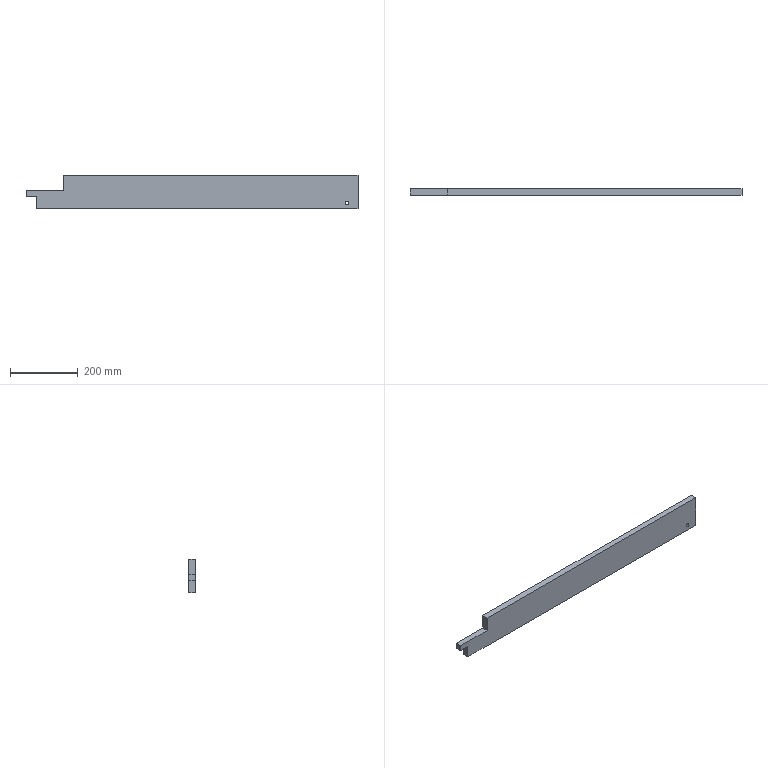Part | STEP file | Superstructure_3 | 1 solid | 11 faces | box 980 x 18 x 100 mm | volume 1653506 mm3 | plane 10 | cylinder 1 | commonest cylinder face diameters 10 x1
STEP:
#1=CARTESIAN_POINT('',(0.,0.,0.));
#2=DIRECTION('',(0.,0.,1.));
#3=DIRECTION('',(1.,0.,0.));
#4=AXIS2_PLACEMENT_3D('',#1,#2,#3);
#5=CARTESIAN_POINT('',(0.,9.,0.));
#6=VERTEX_POINT('',#5);
#7=CARTESIAN_POINT('',(0.,-9.,0.));
#8=VERTEX_POINT('',#7);
#9=CARTESIAN_POINT('',(0.,9.,0.));
#10=DIRECTION('',(0.,-1.,0.));
#11=VECTOR('',#10,1.);
#12=LINE('',#9,#11);
#13=CARTESIAN_POINT('',(0.,9.,0.));
#14=DIRECTION('',(-1.,0.,0.));
#15=DIRECTION('',(0.,0.,1.));
#16=AXIS2_PLACEMENT_3D('',#13,#14,#15);
#17=PLANE('',#16);
#18=CARTESIAN_POINT('',(0.,0.));
#19=DIRECTION('',(0.,-1.));
#20=VECTOR('',#19,1.);
#21=LINE('',#18,#20);
#22=(GEOMETRIC_REPRESENTATION_CONTEXT(2)PARAMETRIC_REPRESENTATION_CONTEXT()REPRESENTATION_CONTEXT('',''));
#23=DEFINITIONAL_REPRESENTATION('',(#21),#22);
#24=PCURVE('',#17,#23);
#25=CARTESIAN_POINT('',(950.,9.,0.));
#26=DIRECTION('',(0.,0.,-1.));
#27=DIRECTION('',(-1.,0.,0.));
#28=AXIS2_PLACEMENT_3D('',#25,#26,#27);
#29=PLANE('',#28);
#30=CARTESIAN_POINT('',(950.,0.));
#31=DIRECTION('',(0.,-1.));
#32=VECTOR('',#31,1.);
#33=LINE('',#30,#32);
#34=(GEOMETRIC_REPRESENTATION_CONTEXT(2)PARAMETRIC_REPRESENTATION_CONTEXT()REPRESENTATION_CONTEXT('',''));
#35=DEFINITIONAL_REPRESENTATION('',(#33),#34);
#36=PCURVE('',#29,#35);
#37=SURFACE_CURVE('',#12,(#24,#36),.PCURVE_S1.);
#38=EDGE_CURVE('',#6,#8,#37,.T.);
#39=ORIENTED_EDGE('',*,*,#38,.T.);
#40=CARTESIAN_POINT('',(0.,-9.,37.));
#41=VERTEX_POINT('',#40);
#42=CARTESIAN_POINT('',(0.,-9.,0.));
#43=DIRECTION('',(0.,0.,1.));
#44=VECTOR('',#43,1.);
#45=LINE('',#42,#44);
#46=CARTESIAN_POINT('',(0.,-18.));
#47=DIRECTION('',(1.,0.));
#48=VECTOR('',#47,1.);
#49=LINE('',#46,#48);
#50=(GEOMETRIC_REPRESENTATION_CONTEXT(2)PARAMETRIC_REPRESENTATION_CONTEXT()REPRESENTATION_CONTEXT('',''));
#51=DEFINITIONAL_REPRESENTATION('',(#49),#50);
#52=PCURVE('',#17,#51);
#53=CARTESIAN_POINT('',(468.21,-9.,47.857));
#54=DIRECTION('',(0.,1.,0.));
#55=DIRECTION('',(0.,0.,1.));
#56=AXIS2_PLACEMENT_3D('',#53,#54,#55);
#57=PLANE('',#56);
#58=CARTESIAN_POINT('',(-47.857,-468.21));
#59=DIRECTION('',(1.,0.));
#60=VECTOR('',#59,1.);
#61=LINE('',#58,#60);
#62=(GEOMETRIC_REPRESENTATION_CONTEXT(2)PARAMETRIC_REPRESENTATION_CONTEXT()REPRESENTATION_CONTEXT('',''));
#63=DEFINITIONAL_REPRESENTATION('',(#61),#62);
#64=PCURVE('',#57,#63);
#65=SURFACE_CURVE('',#45,(#52,#64),.PCURVE_S1.);
#66=EDGE_CURVE('',#8,#41,#65,.T.);
#67=ORIENTED_EDGE('',*,*,#66,.T.);
#68=CARTESIAN_POINT('',(0.,9.,37.));
#69=VERTEX_POINT('',#68);
#70=CARTESIAN_POINT('',(0.,9.,37.));
#71=DIRECTION('',(0.,-1.,0.));
#72=VECTOR('',#71,1.);
#73=LINE('',#70,#72);
#74=CARTESIAN_POINT('',(37.,0.));
#75=DIRECTION('',(0.,-1.));
#76=VECTOR('',#75,1.);
#77=LINE('',#74,#76);
#78=(GEOMETRIC_REPRESENTATION_CONTEXT(2)PARAMETRIC_REPRESENTATION_CONTEXT()REPRESENTATION_CONTEXT('',''));
#79=DEFINITIONAL_REPRESENTATION('',(#77),#78);
#80=PCURVE('',#17,#79);
#81=CARTESIAN_POINT('',(0.,9.,37.));
#82=DIRECTION('',(0.,0.,-1.));
#83=DIRECTION('',(-1.,0.,0.));
#84=AXIS2_PLACEMENT_3D('',#81,#82,#83);
#85=PLANE('',#84);
#86=CARTESIAN_POINT('',(0.,0.));
#87=DIRECTION('',(0.,-1.));
#88=VECTOR('',#87,1.);
#89=LINE('',#86,#88);
#90=(GEOMETRIC_REPRESENTATION_CONTEXT(2)PARAMETRIC_REPRESENTATION_CONTEXT()REPRESENTATION_CONTEXT('',''));
#91=DEFINITIONAL_REPRESENTATION('',(#89),#90);
#92=PCURVE('',#85,#91);
#93=SURFACE_CURVE('',#73,(#80,#92),.PCURVE_S1.);
#94=EDGE_CURVE('',#69,#41,#93,.T.);
#95=ORIENTED_EDGE('',*,*,#94,.F.);
#96=CARTESIAN_POINT('',(0.,9.,0.));
#97=DIRECTION('',(0.,0.,1.));
#98=VECTOR('',#97,1.);
#99=LINE('',#96,#98);
#100=CARTESIAN_POINT('',(0.,0.));
#101=DIRECTION('',(1.,0.));
#102=VECTOR('',#101,1.);
#103=LINE('',#100,#102);
#104=(GEOMETRIC_REPRESENTATION_CONTEXT(2)PARAMETRIC_REPRESENTATION_CONTEXT()REPRESENTATION_CONTEXT('',''));
#105=DEFINITIONAL_REPRESENTATION('',(#103),#104);
#106=PCURVE('',#17,#105);
#107=CARTESIAN_POINT('',(468.21,9.,47.857));
#108=DIRECTION('',(0.,1.,0.));
#109=DIRECTION('',(0.,0.,1.));
#110=AXIS2_PLACEMENT_3D('',#107,#108,#109);
#111=PLANE('',#110);
#112=CARTESIAN_POINT('',(-47.857,-468.21));
#113=DIRECTION('',(1.,0.));
#114=VECTOR('',#113,1.);
#115=LINE('',#112,#114);
#116=(GEOMETRIC_REPRESENTATION_CONTEXT(2)PARAMETRIC_REPRESENTATION_CONTEXT()REPRESENTATION_CONTEXT('',''));
#117=DEFINITIONAL_REPRESENTATION('',(#115),#116);
#118=PCURVE('',#111,#117);
#119=SURFACE_CURVE('',#99,(#106,#118),.PCURVE_S1.);
#120=EDGE_CURVE('',#6,#69,#119,.T.);
#121=ORIENTED_EDGE('',*,*,#120,.F.);
#122=EDGE_LOOP('',(#39,#67,#95,#121));
#123=FACE_BOUND('',#122,.T.);
#124=ADVANCED_FACE('',(#123),#17,.T.);
#125=ORIENTED_EDGE('',*,*,#94,.T.);
#126=CARTESIAN_POINT('',(-30.,-9.,37.));
#127=VERTEX_POINT('',#126);
#128=CARTESIAN_POINT('',(0.,-9.,37.));
#129=DIRECTION('',(-1.,0.,0.));
#130=VECTOR('',#129,1.);
#131=LINE('',#128,#130);
#132=CARTESIAN_POINT('',(0.,-18.));
#133=DIRECTION('',(1.,0.));
#134=VECTOR('',#133,1.);
#135=LINE('',#132,#134);
#136=(GEOMETRIC_REPRESENTATION_CONTEXT(2)PARAMETRIC_REPRESENTATION_CONTEXT()REPRESENTATION_CONTEXT('',''));
#137=DEFINITIONAL_REPRESENTATION('',(#135),#136);
#138=PCURVE('',#85,#137);
#139=CARTESIAN_POINT('',(-10.857,-468.21));
#140=DIRECTION('',(0.,-1.));
#141=VECTOR('',#140,1.);
#142=LINE('',#139,#141);
#143=(GEOMETRIC_REPRESENTATION_CONTEXT(2)PARAMETRIC_REPRESENTATION_CONTEXT()REPRESENTATION_CONTEXT('',''));
#144=DEFINITIONAL_REPRESENTATION('',(#142),#143);
#145=PCURVE('',#57,#144);
#146=SURFACE_CURVE('',#131,(#138,#145),.PCURVE_S1.);
#147=EDGE_CURVE('',#41,#127,#146,.T.);
#148=ORIENTED_EDGE('',*,*,#147,.T.);
#149=CARTESIAN_POINT('',(-30.,9.,37.));
#150=VERTEX_POINT('',#149);
#151=CARTESIAN_POINT('',(-30.,9.,37.));
#152=DIRECTION('',(0.,-1.,0.));
#153=VECTOR('',#152,1.);
#154=LINE('',#151,#153);
#155=CARTESIAN_POINT('',(30.,0.));
#156=DIRECTION('',(0.,-1.));
#157=VECTOR('',#156,1.);
#158=LINE('',#155,#157);
#159=(GEOMETRIC_REPRESENTATION_CONTEXT(2)PARAMETRIC_REPRESENTATION_CONTEXT()REPRESENTATION_CONTEXT('',''));
#160=DEFINITIONAL_REPRESENTATION('',(#158),#159);
#161=PCURVE('',#85,#160);
#162=CARTESIAN_POINT('',(-30.,9.,37.));
#163=DIRECTION('',(-1.,0.,0.));
#164=DIRECTION('',(0.,0.,1.));
#165=AXIS2_PLACEMENT_3D('',#162,#163,#164);
#166=PLANE('',#165);
#167=CARTESIAN_POINT('',(0.,0.));
#168=DIRECTION('',(0.,-1.));
#169=VECTOR('',#168,1.);
#170=LINE('',#167,#169);
#171=(GEOMETRIC_REPRESENTATION_CONTEXT(2)PARAMETRIC_REPRESENTATION_CONTEXT()REPRESENTATION_CONTEXT('',''));
#172=DEFINITIONAL_REPRESENTATION('',(#170),#171);
#173=PCURVE('',#166,#172);
#174=SURFACE_CURVE('',#154,(#161,#173),.PCURVE_S1.);
#175=EDGE_CURVE('',#150,#127,#174,.T.);
#176=ORIENTED_EDGE('',*,*,#175,.F.);
#177=CARTESIAN_POINT('',(0.,9.,37.));
#178=DIRECTION('',(-1.,0.,0.));
#179=VECTOR('',#178,1.);
#180=LINE('',#177,#179);
#181=CARTESIAN_POINT('',(0.,0.));
#182=DIRECTION('',(1.,0.));
#183=VECTOR('',#182,1.);
#184=LINE('',#181,#183);
#185=(GEOMETRIC_REPRESENTATION_CONTEXT(2)PARAMETRIC_REPRESENTATION_CONTEXT()REPRESENTATION_CONTEXT('',''));
#186=DEFINITIONAL_REPRESENTATION('',(#184),#185);
#187=PCURVE('',#85,#186);
#188=CARTESIAN_POINT('',(-10.857,-468.21));
#189=DIRECTION('',(0.,-1.));
#190=VECTOR('',#189,1.);
#191=LINE('',#188,#190);
#192=(GEOMETRIC_REPRESENTATION_CONTEXT(2)PARAMETRIC_REPRESENTATION_CONTEXT()REPRESENTATION_CONTEXT('',''));
#193=DEFINITIONAL_REPRESENTATION('',(#191),#192);
#194=PCURVE('',#111,#193);
#195=SURFACE_CURVE('',#180,(#187,#194),.PCURVE_S1.);
#196=EDGE_CURVE('',#69,#150,#195,.T.);
#197=ORIENTED_EDGE('',*,*,#196,.F.);
#198=EDGE_LOOP('',(#125,#148,#176,#197));
#199=FACE_BOUND('',#198,.T.);
#200=ADVANCED_FACE('',(#199),#85,.T.);
#201=ORIENTED_EDGE('',*,*,#175,.T.);
#202=CARTESIAN_POINT('',(-30.,-9.,55.));
#203=VERTEX_POINT('',#202);
#204=CARTESIAN_POINT('',(-30.,-9.,37.));
#205=DIRECTION('',(0.,0.,1.));
#206=VECTOR('',#205,1.);
#207=LINE('',#204,#206);
#208=CARTESIAN_POINT('',(0.,-18.));
#209=DIRECTION('',(1.,0.));
#210=VECTOR('',#209,1.);
#211=LINE('',#208,#210);
#212=(GEOMETRIC_REPRESENTATION_CONTEXT(2)PARAMETRIC_REPRESENTATION_CONTEXT()REPRESENTATION_CONTEXT('',''));
#213=DEFINITIONAL_REPRESENTATION('',(#211),#212);
#214=PCURVE('',#166,#213);
#215=CARTESIAN_POINT('',(-10.857,-498.21));
#216=DIRECTION('',(1.,0.));
#217=VECTOR('',#216,1.);
#218=LINE('',#215,#217);
#219=(GEOMETRIC_REPRESENTATION_CONTEXT(2)PARAMETRIC_REPRESENTATION_CONTEXT()REPRESENTATION_CONTEXT('',''));
#220=DEFINITIONAL_REPRESENTATION('',(#218),#219);
#221=PCURVE('',#57,#220);
#222=SURFACE_CURVE('',#207,(#214,#221),.PCURVE_S1.);
#223=EDGE_CURVE('',#127,#203,#222,.T.);
#224=ORIENTED_EDGE('',*,*,#223,.T.);
#225=CARTESIAN_POINT('',(-30.,9.,55.));
#226=VERTEX_POINT('',#225);
#227=CARTESIAN_POINT('',(-30.,9.,55.));
#228=DIRECTION('',(0.,-1.,0.));
#229=VECTOR('',#228,1.);
#230=LINE('',#227,#229);
#231=CARTESIAN_POINT('',(18.,0.));
#232=DIRECTION('',(0.,-1.));
#233=VECTOR('',#232,1.);
#234=LINE('',#231,#233);
#235=(GEOMETRIC_REPRESENTATION_CONTEXT(2)PARAMETRIC_REPRESENTATION_CONTEXT()REPRESENTATION_CONTEXT('',''));
#236=DEFINITIONAL_REPRESENTATION('',(#234),#235);
#237=PCURVE('',#166,#236);
#238=CARTESIAN_POINT('',(-30.,9.,55.));
#239=DIRECTION('',(0.,0.,1.));
#240=DIRECTION('',(1.,0.,0.));
#241=AXIS2_PLACEMENT_3D('',#238,#239,#240);
#242=PLANE('',#241);
#243=CARTESIAN_POINT('',(0.,0.));
#244=DIRECTION('',(0.,-1.));
#245=VECTOR('',#244,1.);
#246=LINE('',#243,#245);
#247=(GEOMETRIC_REPRESENTATION_CONTEXT(2)PARAMETRIC_REPRESENTATION_CONTEXT()REPRESENTATION_CONTEXT('',''));
#248=DEFINITIONAL_REPRESENTATION('',(#246),#247);
#249=PCURVE('',#242,#248);
#250=SURFACE_CURVE('',#230,(#237,#249),.PCURVE_S1.);
#251=EDGE_CURVE('',#226,#203,#250,.T.);
#252=ORIENTED_EDGE('',*,*,#251,.F.);
#253=CARTESIAN_POINT('',(-30.,9.,37.));
#254=DIRECTION('',(0.,0.,1.));
#255=VECTOR('',#254,1.);
#256=LINE('',#253,#255);
#257=CARTESIAN_POINT('',(0.,0.));
#258=DIRECTION('',(1.,0.));
#259=VECTOR('',#258,1.);
#260=LINE('',#257,#259);
#261=(GEOMETRIC_REPRESENTATION_CONTEXT(2)PARAMETRIC_REPRESENTATION_CONTEXT()REPRESENTATION_CONTEXT('',''));
#262=DEFINITIONAL_REPRESENTATION('',(#260),#261);
#263=PCURVE('',#166,#262);
#264=CARTESIAN_POINT('',(-10.857,-498.21));
#265=DIRECTION('',(1.,0.));
#266=VECTOR('',#265,1.);
#267=LINE('',#264,#266);
#268=(GEOMETRIC_REPRESENTATION_CONTEXT(2)PARAMETRIC_REPRESENTATION_CONTEXT()REPRESENTATION_CONTEXT('',''));
#269=DEFINITIONAL_REPRESENTATION('',(#267),#268);
#270=PCURVE('',#111,#269);
#271=SURFACE_CURVE('',#256,(#263,#270),.PCURVE_S1.);
#272=EDGE_CURVE('',#150,#226,#271,.T.);
#273=ORIENTED_EDGE('',*,*,#272,.F.);
#274=EDGE_LOOP('',(#201,#224,#252,#273));
#275=FACE_BOUND('',#274,.T.);
#276=ADVANCED_FACE('',(#275),#166,.T.);
#277=ORIENTED_EDGE('',*,*,#251,.T.);
#278=CARTESIAN_POINT('',(80.,-9.,55.));
#279=VERTEX_POINT('',#278);
#280=CARTESIAN_POINT('',(-30.,-9.,55.));
#281=DIRECTION('',(1.,0.,0.));
#282=VECTOR('',#281,1.);
#283=LINE('',#280,#282);
#284=CARTESIAN_POINT('',(0.,-18.));
#285=DIRECTION('',(1.,0.));
#286=VECTOR('',#285,1.);
#287=LINE('',#284,#286);
#288=(GEOMETRIC_REPRESENTATION_CONTEXT(2)PARAMETRIC_REPRESENTATION_CONTEXT()REPRESENTATION_CONTEXT('',''));
#289=DEFINITIONAL_REPRESENTATION('',(#287),#288);
#290=PCURVE('',#242,#289);
#291=CARTESIAN_POINT('',(7.143,-498.21));
#292=DIRECTION('',(0.,1.));
#293=VECTOR('',#292,1.);
#294=LINE('',#291,#293);
#295=(GEOMETRIC_REPRESENTATION_CONTEXT(2)PARAMETRIC_REPRESENTATION_CONTEXT()REPRESENTATION_CONTEXT('',''));
#296=DEFINITIONAL_REPRESENTATION('',(#294),#295);
#297=PCURVE('',#57,#296);
#298=SURFACE_CURVE('',#283,(#290,#297),.PCURVE_S1.);
#299=EDGE_CURVE('',#203,#279,#298,.T.);
#300=ORIENTED_EDGE('',*,*,#299,.T.);
#301=CARTESIAN_POINT('',(80.,9.,55.));
#302=VERTEX_POINT('',#301);
#303=CARTESIAN_POINT('',(80.,9.,55.));
#304=DIRECTION('',(0.,-1.,0.));
#305=VECTOR('',#304,1.);
#306=LINE('',#303,#305);
#307=CARTESIAN_POINT('',(110.,0.));
#308=DIRECTION('',(0.,-1.));
#309=VECTOR('',#308,1.);
#310=LINE('',#307,#309);
#311=(GEOMETRIC_REPRESENTATION_CONTEXT(2)PARAMETRIC_REPRESENTATION_CONTEXT()REPRESENTATION_CONTEXT('',''));
#312=DEFINITIONAL_REPRESENTATION('',(#310),#311);
#313=PCURVE('',#242,#312);
#314=CARTESIAN_POINT('',(80.,9.,55.));
#315=DIRECTION('',(-1.,0.,0.));
#316=DIRECTION('',(0.,0.,1.));
#317=AXIS2_PLACEMENT_3D('',#314,#315,#316);
#318=PLANE('',#317);
#319=CARTESIAN_POINT('',(0.,0.));
#320=DIRECTION('',(0.,-1.));
#321=VECTOR('',#320,1.);
#322=LINE('',#319,#321);
#323=(GEOMETRIC_REPRESENTATION_CONTEXT(2)PARAMETRIC_REPRESENTATION_CONTEXT()REPRESENTATION_CONTEXT('',''));
#324=DEFINITIONAL_REPRESENTATION('',(#322),#323);
#325=PCURVE('',#318,#324);
#326=SURFACE_CURVE('',#306,(#313,#325),.PCURVE_S1.);
#327=EDGE_CURVE('',#302,#279,#326,.T.);
#328=ORIENTED_EDGE('',*,*,#327,.F.);
#329=CARTESIAN_POINT('',(-30.,9.,55.));
#330=DIRECTION('',(1.,0.,0.));
#331=VECTOR('',#330,1.);
#332=LINE('',#329,#331);
#333=CARTESIAN_POINT('',(0.,0.));
#334=DIRECTION('',(1.,0.));
#335=VECTOR('',#334,1.);
#336=LINE('',#333,#335);
#337=(GEOMETRIC_REPRESENTATION_CONTEXT(2)PARAMETRIC_REPRESENTATION_CONTEXT()REPRESENTATION_CONTEXT('',''));
#338=DEFINITIONAL_REPRESENTATION('',(#336),#337);
#339=PCURVE('',#242,#338);
#340=CARTESIAN_POINT('',(7.143,-498.21));
#341=DIRECTION('',(0.,1.));
#342=VECTOR('',#341,1.);
#343=LINE('',#340,#342);
#344=(GEOMETRIC_REPRESENTATION_CONTEXT(2)PARAMETRIC_REPRESENTATION_CONTEXT()REPRESENTATION_CONTEXT('',''));
#345=DEFINITIONAL_REPRESENTATION('',(#343),#344);
#346=PCURVE('',#111,#345);
#347=SURFACE_CURVE('',#332,(#339,#346),.PCURVE_S1.);
#348=EDGE_CURVE('',#226,#302,#347,.T.);
#349=ORIENTED_EDGE('',*,*,#348,.F.);
#350=EDGE_LOOP('',(#277,#300,#328,#349));
#351=FACE_BOUND('',#350,.T.);
#352=ADVANCED_FACE('',(#351),#242,.T.);
#353=ORIENTED_EDGE('',*,*,#327,.T.);
#354=CARTESIAN_POINT('',(80.,-9.,100.));
#355=VERTEX_POINT('',#354);
#356=CARTESIAN_POINT('',(80.,-9.,55.));
#357=DIRECTION('',(0.,0.,1.));
#358=VECTOR('',#357,1.);
#359=LINE('',#356,#358);
#360=CARTESIAN_POINT('',(0.,-18.));
#361=DIRECTION('',(1.,0.));
#362=VECTOR('',#361,1.);
#363=LINE('',#360,#362);
#364=(GEOMETRIC_REPRESENTATION_CONTEXT(2)PARAMETRIC_REPRESENTATION_CONTEXT()REPRESENTATION_CONTEXT('',''));
#365=DEFINITIONAL_REPRESENTATION('',(#363),#364);
#366=PCURVE('',#318,#365);
#367=CARTESIAN_POINT('',(7.143,-388.21));
#368=DIRECTION('',(1.,0.));
#369=VECTOR('',#368,1.);
#370=LINE('',#367,#369);
#371=(GEOMETRIC_REPRESENTATION_CONTEXT(2)PARAMETRIC_REPRESENTATION_CONTEXT()REPRESENTATION_CONTEXT('',''));
#372=DEFINITIONAL_REPRESENTATION('',(#370),#371);
#373=PCURVE('',#57,#372);
#374=SURFACE_CURVE('',#359,(#366,#373),.PCURVE_S1.);
#375=EDGE_CURVE('',#279,#355,#374,.T.);
#376=ORIENTED_EDGE('',*,*,#375,.T.);
#377=CARTESIAN_POINT('',(80.,9.,100.));
#378=VERTEX_POINT('',#377);
#379=CARTESIAN_POINT('',(80.,9.,100.));
#380=DIRECTION('',(0.,-1.,0.));
#381=VECTOR('',#380,1.);
#382=LINE('',#379,#381);
#383=CARTESIAN_POINT('',(45.,0.));
#384=DIRECTION('',(0.,-1.));
#385=VECTOR('',#384,1.);
#386=LINE('',#383,#385);
#387=(GEOMETRIC_REPRESENTATION_CONTEXT(2)PARAMETRIC_REPRESENTATION_CONTEXT()REPRESENTATION_CONTEXT('',''));
#388=DEFINITIONAL_REPRESENTATION('',(#386),#387);
#389=PCURVE('',#318,#388);
#390=CARTESIAN_POINT('',(80.,9.,100.));
#391=DIRECTION('',(0.,0.,1.));
#392=DIRECTION('',(1.,0.,0.));
#393=AXIS2_PLACEMENT_3D('',#390,#391,#392);
#394=PLANE('',#393);
#395=CARTESIAN_POINT('',(0.,0.));
#396=DIRECTION('',(0.,-1.));
#397=VECTOR('',#396,1.);
#398=LINE('',#395,#397);
#399=(GEOMETRIC_REPRESENTATION_CONTEXT(2)PARAMETRIC_REPRESENTATION_CONTEXT()REPRESENTATION_CONTEXT('',''));
#400=DEFINITIONAL_REPRESENTATION('',(#398),#399);
#401=PCURVE('',#394,#400);
#402=SURFACE_CURVE('',#382,(#389,#401),.PCURVE_S1.);
#403=EDGE_CURVE('',#378,#355,#402,.T.);
#404=ORIENTED_EDGE('',*,*,#403,.F.);
#405=CARTESIAN_POINT('',(80.,9.,55.));
#406=DIRECTION('',(0.,0.,1.));
#407=VECTOR('',#406,1.);
#408=LINE('',#405,#407);
#409=CARTESIAN_POINT('',(0.,0.));
#410=DIRECTION('',(1.,0.));
#411=VECTOR('',#410,1.);
#412=LINE('',#409,#411);
#413=(GEOMETRIC_REPRESENTATION_CONTEXT(2)PARAMETRIC_REPRESENTATION_CONTEXT()REPRESENTATION_CONTEXT('',''));
#414=DEFINITIONAL_REPRESENTATION('',(#412),#413);
#415=PCURVE('',#318,#414);
#416=CARTESIAN_POINT('',(7.143,-388.21));
#417=DIRECTION('',(1.,0.));
#418=VECTOR('',#417,1.);
#419=LINE('',#416,#418);
#420=(GEOMETRIC_REPRESENTATION_CONTEXT(2)PARAMETRIC_REPRESENTATION_CONTEXT()REPRESENTATION_CONTEXT('',''));
#421=DEFINITIONAL_REPRESENTATION('',(#419),#420);
#422=PCURVE('',#111,#421);
#423=SURFACE_CURVE('',#408,(#415,#422),.PCURVE_S1.);
#424=EDGE_CURVE('',#302,#378,#423,.T.);
#425=ORIENTED_EDGE('',*,*,#424,.F.);
#426=EDGE_LOOP('',(#353,#376,#404,#425));
#427=FACE_BOUND('',#426,.T.);
#428=ADVANCED_FACE('',(#427),#318,.T.);
#429=ORIENTED_EDGE('',*,*,#403,.T.);
#430=CARTESIAN_POINT('',(950.,-9.,100.));
#431=VERTEX_POINT('',#430);
#432=CARTESIAN_POINT('',(80.,-9.,100.));
#433=DIRECTION('',(1.,0.,0.));
#434=VECTOR('',#433,1.);
#435=LINE('',#432,#434);
#436=CARTESIAN_POINT('',(0.,-18.));
#437=DIRECTION('',(1.,0.));
#438=VECTOR('',#437,1.);
#439=LINE('',#436,#438);
#440=(GEOMETRIC_REPRESENTATION_CONTEXT(2)PARAMETRIC_REPRESENTATION_CONTEXT()REPRESENTATION_CONTEXT('',''));
#441=DEFINITIONAL_REPRESENTATION('',(#439),#440);
#442=PCURVE('',#394,#441);
#443=CARTESIAN_POINT('',(52.143,-388.21));
#444=DIRECTION('',(0.,1.));
#445=VECTOR('',#444,1.);
#446=LINE('',#443,#445);
#447=(GEOMETRIC_REPRESENTATION_CONTEXT(2)PARAMETRIC_REPRESENTATION_CONTEXT()REPRESENTATION_CONTEXT('',''));
#448=DEFINITIONAL_REPRESENTATION('',(#446),#447);
#449=PCURVE('',#57,#448);
#450=SURFACE_CURVE('',#435,(#442,#449),.PCURVE_S1.);
#451=EDGE_CURVE('',#355,#431,#450,.T.);
#452=ORIENTED_EDGE('',*,*,#451,.T.);
#453=CARTESIAN_POINT('',(950.,9.,100.));
#454=VERTEX_POINT('',#453);
#455=CARTESIAN_POINT('',(950.,9.,100.));
#456=DIRECTION('',(0.,-1.,0.));
#457=VECTOR('',#456,1.);
#458=LINE('',#455,#457);
#459=CARTESIAN_POINT('',(870.,0.));
#460=DIRECTION('',(0.,-1.));
#461=VECTOR('',#460,1.);
#462=LINE('',#459,#461);
#463=(GEOMETRIC_REPRESENTATION_CONTEXT(2)PARAMETRIC_REPRESENTATION_CONTEXT()REPRESENTATION_CONTEXT('',''));
#464=DEFINITIONAL_REPRESENTATION('',(#462),#463);
#465=PCURVE('',#394,#464);
#466=CARTESIAN_POINT('',(950.,9.,100.));
#467=DIRECTION('',(1.,0.,0.));
#468=DIRECTION('',(0.,0.,-1.));
#469=AXIS2_PLACEMENT_3D('',#466,#467,#468);
#470=PLANE('',#469);
#471=CARTESIAN_POINT('',(0.,0.));
#472=DIRECTION('',(0.,-1.));
#473=VECTOR('',#472,1.);
#474=LINE('',#471,#473);
#475=(GEOMETRIC_REPRESENTATION_CONTEXT(2)PARAMETRIC_REPRESENTATION_CONTEXT()REPRESENTATION_CONTEXT('',''));
#476=DEFINITIONAL_REPRESENTATION('',(#474),#475);
#477=PCURVE('',#470,#476);
#478=SURFACE_CURVE('',#458,(#465,#477),.PCURVE_S1.);
#479=EDGE_CURVE('',#454,#431,#478,.T.);
#480=ORIENTED_EDGE('',*,*,#479,.F.);
#481=CARTESIAN_POINT('',(80.,9.,100.));
#482=DIRECTION('',(1.,0.,0.));
#483=VECTOR('',#482,1.);
#484=LINE('',#481,#483);
#485=CARTESIAN_POINT('',(0.,0.));
#486=DIRECTION('',(1.,0.));
#487=VECTOR('',#486,1.);
#488=LINE('',#485,#487);
#489=(GEOMETRIC_REPRESENTATION_CONTEXT(2)PARAMETRIC_REPRESENTATION_CONTEXT()REPRESENTATION_CONTEXT('',''));
#490=DEFINITIONAL_REPRESENTATION('',(#488),#489);
#491=PCURVE('',#394,#490);
#492=CARTESIAN_POINT('',(52.143,-388.21));
#493=DIRECTION('',(0.,1.));
#494=VECTOR('',#493,1.);
#495=LINE('',#492,#494);
#496=(GEOMETRIC_REPRESENTATION_CONTEXT(2)PARAMETRIC_REPRESENTATION_CONTEXT()REPRESENTATION_CONTEXT('',''));
#497=DEFINITIONAL_REPRESENTATION('',(#495),#496);
#498=PCURVE('',#111,#497);
#499=SURFACE_CURVE('',#484,(#491,#498),.PCURVE_S1.);
#500=EDGE_CURVE('',#378,#454,#499,.T.);
#501=ORIENTED_EDGE('',*,*,#500,.F.);
#502=EDGE_LOOP('',(#429,#452,#480,#501));
#503=FACE_BOUND('',#502,.T.);
#504=ADVANCED_FACE('',(#503),#394,.T.);
#505=ORIENTED_EDGE('',*,*,#479,.T.);
#506=CARTESIAN_POINT('',(950.,-9.,0.));
#507=VERTEX_POINT('',#506);
#508=CARTESIAN_POINT('',(950.,-9.,100.));
#509=DIRECTION('',(0.,0.,-1.));
#510=VECTOR('',#509,1.);
#511=LINE('',#508,#510);
#512=CARTESIAN_POINT('',(0.,-18.));
#513=DIRECTION('',(1.,0.));
#514=VECTOR('',#513,1.);
#515=LINE('',#512,#514);
#516=(GEOMETRIC_REPRESENTATION_CONTEXT(2)PARAMETRIC_REPRESENTATION_CONTEXT()REPRESENTATION_CONTEXT('',''));
#517=DEFINITIONAL_REPRESENTATION('',(#515),#516);
#518=PCURVE('',#470,#517);
#519=CARTESIAN_POINT('',(52.143,481.79));
#520=DIRECTION('',(-1.,0.));
#521=VECTOR('',#520,1.);
#522=LINE('',#519,#521);
#523=(GEOMETRIC_REPRESENTATION_CONTEXT(2)PARAMETRIC_REPRESENTATION_CONTEXT()REPRESENTATION_CONTEXT('',''));
#524=DEFINITIONAL_REPRESENTATION('',(#522),#523);
#525=PCURVE('',#57,#524);
#526=SURFACE_CURVE('',#511,(#518,#525),.PCURVE_S1.);
#527=EDGE_CURVE('',#431,#507,#526,.T.);
#528=ORIENTED_EDGE('',*,*,#527,.T.);
#529=CARTESIAN_POINT('',(950.,9.,0.));
#530=VERTEX_POINT('',#529);
#531=CARTESIAN_POINT('',(950.,9.,0.));
#532=DIRECTION('',(0.,-1.,0.));
#533=VECTOR('',#532,1.);
#534=LINE('',#531,#533);
#535=CARTESIAN_POINT('',(100.,0.));
#536=DIRECTION('',(0.,-1.));
#537=VECTOR('',#536,1.);
#538=LINE('',#535,#537);
#539=(GEOMETRIC_REPRESENTATION_CONTEXT(2)PARAMETRIC_REPRESENTATION_CONTEXT()REPRESENTATION_CONTEXT('',''));
#540=DEFINITIONAL_REPRESENTATION('',(#538),#539);
#541=PCURVE('',#470,#540);
#542=CARTESIAN_POINT('',(0.,0.));
#543=DIRECTION('',(0.,-1.));
#544=VECTOR('',#543,1.);
#545=LINE('',#542,#544);
#546=(GEOMETRIC_REPRESENTATION_CONTEXT(2)PARAMETRIC_REPRESENTATION_CONTEXT()REPRESENTATION_CONTEXT('',''));
#547=DEFINITIONAL_REPRESENTATION('',(#545),#546);
#548=PCURVE('',#29,#547);
#549=SURFACE_CURVE('',#534,(#541,#548),.PCURVE_S1.);
#550=EDGE_CURVE('',#530,#507,#549,.T.);
#551=ORIENTED_EDGE('',*,*,#550,.F.);
#552=CARTESIAN_POINT('',(950.,9.,100.));
#553=DIRECTION('',(0.,0.,-1.));
#554=VECTOR('',#553,1.);
#555=LINE('',#552,#554);
#556=CARTESIAN_POINT('',(0.,0.));
#557=DIRECTION('',(1.,0.));
#558=VECTOR('',#557,1.);
#559=LINE('',#556,#558);
#560=(GEOMETRIC_REPRESENTATION_CONTEXT(2)PARAMETRIC_REPRESENTATION_CONTEXT()REPRESENTATION_CONTEXT('',''));
#561=DEFINITIONAL_REPRESENTATION('',(#559),#560);
#562=PCURVE('',#470,#561);
#563=CARTESIAN_POINT('',(52.143,481.79));
#564=DIRECTION('',(-1.,0.));
#565=VECTOR('',#564,1.);
#566=LINE('',#563,#565);
#567=(GEOMETRIC_REPRESENTATION_CONTEXT(2)PARAMETRIC_REPRESENTATION_CONTEXT()REPRESENTATION_CONTEXT('',''));
#568=DEFINITIONAL_REPRESENTATION('',(#566),#567);
#569=PCURVE('',#111,#568);
#570=SURFACE_CURVE('',#555,(#562,#569),.PCURVE_S1.);
#571=EDGE_CURVE('',#454,#530,#570,.T.);
#572=ORIENTED_EDGE('',*,*,#571,.F.);
#573=EDGE_LOOP('',(#505,#528,#551,#572));
#574=FACE_BOUND('',#573,.T.);
#575=ADVANCED_FACE('',(#574),#470,.T.);
#576=ORIENTED_EDGE('',*,*,#550,.T.);
#577=CARTESIAN_POINT('',(950.,-9.,0.));
#578=DIRECTION('',(-1.,0.,0.));
#579=VECTOR('',#578,1.);
#580=LINE('',#577,#579);
#581=CARTESIAN_POINT('',(0.,-18.));
#582=DIRECTION('',(1.,0.));
#583=VECTOR('',#582,1.);
#584=LINE('',#581,#583);
#585=(GEOMETRIC_REPRESENTATION_CONTEXT(2)PARAMETRIC_REPRESENTATION_CONTEXT()REPRESENTATION_CONTEXT('',''));
#586=DEFINITIONAL_REPRESENTATION('',(#584),#585);
#587=PCURVE('',#29,#586);
#588=CARTESIAN_POINT('',(-47.857,481.79));
#589=DIRECTION('',(0.,-1.));
#590=VECTOR('',#589,1.);
#591=LINE('',#588,#590);
#592=(GEOMETRIC_REPRESENTATION_CONTEXT(2)PARAMETRIC_REPRESENTATION_CONTEXT()REPRESENTATION_CONTEXT('',''));
#593=DEFINITIONAL_REPRESENTATION('',(#591),#592);
#594=PCURVE('',#57,#593);
#595=SURFACE_CURVE('',#580,(#587,#594),.PCURVE_S1.);
#596=EDGE_CURVE('',#507,#8,#595,.T.);
#597=ORIENTED_EDGE('',*,*,#596,.T.);
#598=ORIENTED_EDGE('',*,*,#38,.F.);
#599=CARTESIAN_POINT('',(950.,9.,0.));
#600=DIRECTION('',(-1.,0.,0.));
#601=VECTOR('',#600,1.);
#602=LINE('',#599,#601);
#603=CARTESIAN_POINT('',(0.,0.));
#604=DIRECTION('',(1.,0.));
#605=VECTOR('',#604,1.);
#606=LINE('',#603,#605);
#607=(GEOMETRIC_REPRESENTATION_CONTEXT(2)PARAMETRIC_REPRESENTATION_CONTEXT()REPRESENTATION_CONTEXT('',''));
#608=DEFINITIONAL_REPRESENTATION('',(#606),#607);
#609=PCURVE('',#29,#608);
#610=CARTESIAN_POINT('',(-47.857,481.79));
#611=DIRECTION('',(0.,-1.));
#612=VECTOR('',#611,1.);
#613=LINE('',#610,#612);
#614=(GEOMETRIC_REPRESENTATION_CONTEXT(2)PARAMETRIC_REPRESENTATION_CONTEXT()REPRESENTATION_CONTEXT('',''));
#615=DEFINITIONAL_REPRESENTATION('',(#613),#614);
#616=PCURVE('',#111,#615);
#617=SURFACE_CURVE('',#602,(#609,#616),.PCURVE_S1.);
#618=EDGE_CURVE('',#530,#6,#617,.T.);
#619=ORIENTED_EDGE('',*,*,#618,.F.);
#620=EDGE_LOOP('',(#576,#597,#598,#619));
#621=FACE_BOUND('',#620,.T.);
#622=ADVANCED_FACE('',(#621),#29,.T.);
#623=CARTESIAN_POINT('',(922.5,9.,17.5));
#624=VERTEX_POINT('',#623);
#625=CARTESIAN_POINT('',(917.5,9.,17.5));
#626=DIRECTION('',(0.,-1.,0.));
#627=DIRECTION('',(1.,0.,0.));
#628=AXIS2_PLACEMENT_3D('',#625,#626,#627);
#629=CIRCLE('',#628,5.);
#630=CARTESIAN_POINT('',(917.5,9.,17.5));
#631=DIRECTION('',(0.,1.,0.));
#632=DIRECTION('',(1.,0.,0.));
#633=AXIS2_PLACEMENT_3D('',#630,#631,#632);
#634=CYLINDRICAL_SURFACE('',#633,5.);
#635=CARTESIAN_POINT('',(6.283,0.));
#636=DIRECTION('',(-1.,0.));
#637=VECTOR('',#636,1.);
#638=LINE('',#635,#637);
#639=(GEOMETRIC_REPRESENTATION_CONTEXT(2)PARAMETRIC_REPRESENTATION_CONTEXT()REPRESENTATION_CONTEXT('',''));
#640=DEFINITIONAL_REPRESENTATION('',(#638),#639);
#641=PCURVE('',#634,#640);
#642=CARTESIAN_POINT('',(-30.357,454.29));
#643=CARTESIAN_POINT('',(-21.697,454.29));
#644=CARTESIAN_POINT('',(-26.027,446.79));
#645=CARTESIAN_POINT('',(-30.357,439.29));
#646=CARTESIAN_POINT('',(-34.687,446.79));
#647=CARTESIAN_POINT('',(-39.017,454.29));
#648=CARTESIAN_POINT('',(-30.357,454.29));
#649=(BOUNDED_CURVE()B_SPLINE_CURVE(2,(#642,#643,#644,#645,#646,#647,#648),.UNSPECIFIED.,.T.,.F.)B_SPLINE_CURVE_WITH_KNOTS((1,2,2,2,2,1),(-2.094,0.,2.094,4.189,6.283,8.378),.UNSPECIFIED.)CURVE()GEOMETRIC_REPRESENTATION_ITEM()RATIONAL_B_SPLINE_CURVE((1.,0.5,1.,0.5,1.,0.5,1.))REPRESENTATION_ITEM(''));
#650=(GEOMETRIC_REPRESENTATION_CONTEXT(2)PARAMETRIC_REPRESENTATION_CONTEXT()REPRESENTATION_CONTEXT('',''));
#651=DEFINITIONAL_REPRESENTATION('',(#649),#650);
#652=PCURVE('',#111,#651);
#653=SURFACE_CURVE('',#629,(#641,#652),.PCURVE_S1.);
#654=EDGE_CURVE('',#624,#624,#653,.T.);
#655=ORIENTED_EDGE('',*,*,#654,.T.);
#656=CARTESIAN_POINT('',(922.5,-9.,17.5));
#657=VERTEX_POINT('',#656);
#658=CARTESIAN_POINT('',(922.5,9.,17.5));
#659=DIRECTION('',(0.,-1.,0.));
#660=VECTOR('',#659,1.);
#661=LINE('',#658,#660);
#662=CARTESIAN_POINT('',(0.,0.));
#663=DIRECTION('',(0.,-1.));
#664=VECTOR('',#663,1.);
#665=LINE('',#662,#664);
#666=(GEOMETRIC_REPRESENTATION_CONTEXT(2)PARAMETRIC_REPRESENTATION_CONTEXT()REPRESENTATION_CONTEXT('',''));
#667=DEFINITIONAL_REPRESENTATION('',(#665),#666);
#668=PCURVE('',#634,#667);
#669=CARTESIAN_POINT('',(6.283,0.));
#670=DIRECTION('',(0.,-1.));
#671=VECTOR('',#670,1.);
#672=LINE('',#669,#671);
#673=(GEOMETRIC_REPRESENTATION_CONTEXT(2)PARAMETRIC_REPRESENTATION_CONTEXT()REPRESENTATION_CONTEXT('',''));
#674=DEFINITIONAL_REPRESENTATION('',(#672),#673);
#675=PCURVE('',#634,#674);
#676=SEAM_CURVE('',#661,(#668,#675),.PCURVE_S1.);
#677=EDGE_CURVE('',#624,#657,#676,.T.);
#678=ORIENTED_EDGE('',*,*,#677,.T.);
#679=CARTESIAN_POINT('',(917.5,-9.,17.5));
#680=DIRECTION('',(0.,-1.,0.));
#681=DIRECTION('',(1.,0.,0.));
#682=AXIS2_PLACEMENT_3D('',#679,#680,#681);
#683=CIRCLE('',#682,5.);
#684=CARTESIAN_POINT('',(6.283,-18.));
#685=DIRECTION('',(-1.,0.));
#686=VECTOR('',#685,1.);
#687=LINE('',#684,#686);
#688=(GEOMETRIC_REPRESENTATION_CONTEXT(2)PARAMETRIC_REPRESENTATION_CONTEXT()REPRESENTATION_CONTEXT('',''));
#689=DEFINITIONAL_REPRESENTATION('',(#687),#688);
#690=PCURVE('',#634,#689);
#691=CARTESIAN_POINT('',(-30.357,454.29));
#692=CARTESIAN_POINT('',(-21.697,454.29));
#693=CARTESIAN_POINT('',(-26.027,446.79));
#694=CARTESIAN_POINT('',(-30.357,439.29));
#695=CARTESIAN_POINT('',(-34.687,446.79));
#696=CARTESIAN_POINT('',(-39.017,454.29));
#697=CARTESIAN_POINT('',(-30.357,454.29));
#698=(BOUNDED_CURVE()B_SPLINE_CURVE(2,(#691,#692,#693,#694,#695,#696,#697),.UNSPECIFIED.,.T.,.F.)B_SPLINE_CURVE_WITH_KNOTS((1,2,2,2,2,1),(-2.094,0.,2.094,4.189,6.283,8.378),.UNSPECIFIED.)CURVE()GEOMETRIC_REPRESENTATION_ITEM()RATIONAL_B_SPLINE_CURVE((1.,0.5,1.,0.5,1.,0.5,1.))REPRESENTATION_ITEM(''));
#699=(GEOMETRIC_REPRESENTATION_CONTEXT(2)PARAMETRIC_REPRESENTATION_CONTEXT()REPRESENTATION_CONTEXT('',''));
#700=DEFINITIONAL_REPRESENTATION('',(#698),#699);
#701=PCURVE('',#57,#700);
#702=SURFACE_CURVE('',#683,(#690,#701),.PCURVE_S1.);
#703=EDGE_CURVE('',#657,#657,#702,.T.);
#704=ORIENTED_EDGE('',*,*,#703,.F.);
#705=ORIENTED_EDGE('',*,*,#677,.F.);
#706=EDGE_LOOP('',(#655,#678,#704,#705));
#707=FACE_BOUND('',#706,.F.);
#708=ADVANCED_FACE('',(#707),#634,.F.);
#709=ORIENTED_EDGE('',*,*,#120,.T.);
#710=ORIENTED_EDGE('',*,*,#196,.T.);
#711=ORIENTED_EDGE('',*,*,#272,.T.);
#712=ORIENTED_EDGE('',*,*,#348,.T.);
#713=ORIENTED_EDGE('',*,*,#424,.T.);
#714=ORIENTED_EDGE('',*,*,#500,.T.);
#715=ORIENTED_EDGE('',*,*,#571,.T.);
#716=ORIENTED_EDGE('',*,*,#618,.T.);
#717=EDGE_LOOP('',(#709,#710,#711,#712,#713,#714,#715,#716));
#718=FACE_BOUND('',#717,.T.);
#719=ORIENTED_EDGE('',*,*,#654,.T.);
#720=EDGE_LOOP('',(#719));
#721=FACE_BOUND('',#720,.T.);
#722=ADVANCED_FACE('',(#718,#721),#111,.T.);
#723=ORIENTED_EDGE('',*,*,#66,.T.);
#724=ORIENTED_EDGE('',*,*,#147,.T.);
#725=ORIENTED_EDGE('',*,*,#223,.T.);
#726=ORIENTED_EDGE('',*,*,#299,.T.);
#727=ORIENTED_EDGE('',*,*,#375,.T.);
#728=ORIENTED_EDGE('',*,*,#451,.T.);
#729=ORIENTED_EDGE('',*,*,#527,.T.);
#730=ORIENTED_EDGE('',*,*,#596,.T.);
#731=EDGE_LOOP('',(#723,#724,#725,#726,#727,#728,#729,#730));
#732=FACE_BOUND('',#731,.F.);
#733=ORIENTED_EDGE('',*,*,#703,.T.);
#734=EDGE_LOOP('',(#733));
#735=FACE_BOUND('',#734,.F.);
#736=ADVANCED_FACE('',(#732,#735),#57,.F.);
#737=CLOSED_SHELL('',(#124,#200,#276,#352,#428,#504,#575,#622,#708,#722,#736));
#738=MANIFOLD_SOLID_BREP('',#737);
#739=(LENGTH_UNIT()NAMED_UNIT(*)SI_UNIT(.MILLI.,.METRE.));
#740=UNCERTAINTY_MEASURE_WITH_UNIT(LENGTH_MEASURE(0.0000001),#739,'','');
#741=(NAMED_UNIT(*)PLANE_ANGLE_UNIT()SI_UNIT($,.RADIAN.));
#742=(NAMED_UNIT(*)SI_UNIT($,.STERADIAN.)SOLID_ANGLE_UNIT());
#743=(GEOMETRIC_REPRESENTATION_CONTEXT(3)GLOBAL_UNCERTAINTY_ASSIGNED_CONTEXT((#740))GLOBAL_UNIT_ASSIGNED_CONTEXT((#739,#741,#742))REPRESENTATION_CONTEXT('',''));
#744=ADVANCED_BREP_SHAPE_REPRESENTATION('',(#4,#738),#743);